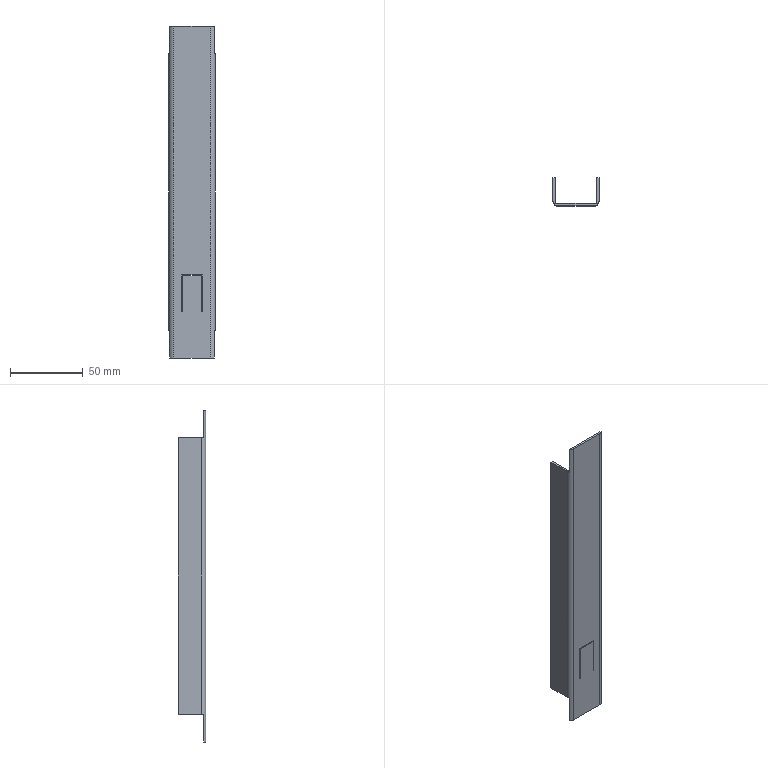Part | SolidWorks | features ICE 2, Extrusion 1 | 1 solid | 26 faces | box 31.75 x 19.05 x 228.6 mm | volume 20094 mm3 | plane 22 | cylinder 4 | commonest cylinder face diameters 3.2 x2 6.4 x2
STEP:
#1=CARTESIAN_POINT('',(31.261,1.5,228.6));
#2=VERTEX_POINT('',#1);
#3=CARTESIAN_POINT('',(0.4889,1.5,228.6));
#4=VERTEX_POINT('',#3);
#5=CARTESIAN_POINT('',(3.1,1.5,228.6));
#6=DIRECTION('',(-1.,0.,0.));
#7=VECTOR('',#6,1000.);
#8=LINE('',#5,#7);
#9=EDGE_CURVE('',#2,#4,#8,.T.);
#10=ORIENTED_EDGE('',*,*,#9,.F.);
#11=CARTESIAN_POINT('',(31.261,1.5,209.55));
#12=VERTEX_POINT('',#11);
#13=CARTESIAN_POINT('',(31.261,1.5,228.6));
#14=DIRECTION('',(0.,0.,-1.));
#15=VECTOR('',#14,1000.);
#16=LINE('',#13,#15);
#17=EDGE_CURVE('',#2,#12,#16,.T.);
#18=ORIENTED_EDGE('',*,*,#17,.T.);
#19=CARTESIAN_POINT('',(28.65,1.5,209.55));
#20=VERTEX_POINT('',#19);
#21=CARTESIAN_POINT('',(31.75,1.5,209.55));
#22=DIRECTION('',(-1.,0.,0.));
#23=VECTOR('',#22,1000.);
#24=LINE('',#21,#23);
#25=EDGE_CURVE('',#12,#20,#24,.T.);
#26=ORIENTED_EDGE('',*,*,#25,.T.);
#27=CARTESIAN_POINT('',(28.65,1.5,19.05));
#28=VERTEX_POINT('',#27);
#29=CARTESIAN_POINT('',(28.65,1.5,228.6));
#30=DIRECTION('',(0.,0.,-1.));
#31=VECTOR('',#30,1000.);
#32=LINE('',#29,#31);
#33=EDGE_CURVE('',#20,#28,#32,.T.);
#34=ORIENTED_EDGE('',*,*,#33,.T.);
#35=CARTESIAN_POINT('',(31.261,1.5,19.05));
#36=VERTEX_POINT('',#35);
#37=CARTESIAN_POINT('',(31.75,1.5,19.05));
#38=DIRECTION('',(-1.,0.,0.));
#39=VECTOR('',#38,1000.);
#40=LINE('',#37,#39);
#41=EDGE_CURVE('',#36,#28,#40,.T.);
#42=ORIENTED_EDGE('',*,*,#41,.F.);
#43=CARTESIAN_POINT('',(31.261,1.5,0.));
#44=VERTEX_POINT('',#43);
#45=CARTESIAN_POINT('',(31.261,1.5,228.6));
#46=DIRECTION('',(0.,0.,-1.));
#47=VECTOR('',#46,1000.);
#48=LINE('',#45,#47);
#49=EDGE_CURVE('',#36,#44,#48,.T.);
#50=ORIENTED_EDGE('',*,*,#49,.T.);
#51=CARTESIAN_POINT('',(0.4889,1.5,0.));
#52=VERTEX_POINT('',#51);
#53=CARTESIAN_POINT('',(3.1,1.5,0.));
#54=DIRECTION('',(-1.,0.,0.));
#55=VECTOR('',#54,1000.);
#56=LINE('',#53,#55);
#57=EDGE_CURVE('',#44,#52,#56,.T.);
#58=ORIENTED_EDGE('',*,*,#57,.T.);
#59=CARTESIAN_POINT('',(0.4889,1.5,19.05));
#60=VERTEX_POINT('',#59);
#61=CARTESIAN_POINT('',(0.4889,1.5,228.6));
#62=DIRECTION('',(0.,0.,1.));
#63=VECTOR('',#62,1000.);
#64=LINE('',#61,#63);
#65=EDGE_CURVE('',#52,#60,#64,.T.);
#66=ORIENTED_EDGE('',*,*,#65,.T.);
#67=CARTESIAN_POINT('',(3.1,1.5,19.05));
#68=VERTEX_POINT('',#67);
#69=CARTESIAN_POINT('',(31.75,1.5,19.05));
#70=DIRECTION('',(-1.,0.,0.));
#71=VECTOR('',#70,1000.);
#72=LINE('',#69,#71);
#73=EDGE_CURVE('',#68,#60,#72,.T.);
#74=ORIENTED_EDGE('',*,*,#73,.F.);
#75=CARTESIAN_POINT('',(3.1,1.5,209.55));
#76=VERTEX_POINT('',#75);
#77=CARTESIAN_POINT('',(3.1,1.5,228.6));
#78=DIRECTION('',(0.,0.,-1.));
#79=VECTOR('',#78,1000.);
#80=LINE('',#77,#79);
#81=EDGE_CURVE('',#76,#68,#80,.T.);
#82=ORIENTED_EDGE('',*,*,#81,.F.);
#83=CARTESIAN_POINT('',(0.4889,1.5,209.55));
#84=VERTEX_POINT('',#83);
#85=CARTESIAN_POINT('',(31.75,1.5,209.55));
#86=DIRECTION('',(-1.,0.,0.));
#87=VECTOR('',#86,1000.);
#88=LINE('',#85,#87);
#89=EDGE_CURVE('',#76,#84,#88,.T.);
#90=ORIENTED_EDGE('',*,*,#89,.T.);
#91=CARTESIAN_POINT('',(0.4889,1.5,228.6));
#92=DIRECTION('',(0.,0.,1.));
#93=VECTOR('',#92,1000.);
#94=LINE('',#91,#93);
#95=EDGE_CURVE('',#84,#4,#94,.T.);
#96=ORIENTED_EDGE('',*,*,#95,.T.);
#97=EDGE_LOOP('',(#10,#18,#26,#34,#42,#50,#58,#66,#74,#82,#90,#96));
#98=FACE_OUTER_BOUND('',#97,.T.);
#99=CARTESIAN_POINT('',(9.428,1.5,31.75));
#100=VERTEX_POINT('',#99);
#101=CARTESIAN_POINT('',(8.928,1.5,31.75));
#102=VERTEX_POINT('',#101);
#103=CARTESIAN_POINT('',(3.1,1.5,31.75));
#104=DIRECTION('',(-1.,0.,0.));
#105=VECTOR('',#104,1000.);
#106=LINE('',#103,#105);
#107=EDGE_CURVE('',#100,#102,#106,.T.);
#108=ORIENTED_EDGE('',*,*,#107,.F.);
#109=CARTESIAN_POINT('',(9.428,1.5,56.65));
#110=VERTEX_POINT('',#109);
#111=CARTESIAN_POINT('',(9.428,1.5,228.6));
#112=DIRECTION('',(0.,0.,-1.));
#113=VECTOR('',#112,1000.);
#114=LINE('',#111,#113);
#115=EDGE_CURVE('',#110,#100,#114,.T.);
#116=ORIENTED_EDGE('',*,*,#115,.F.);
#117=CARTESIAN_POINT('',(22.322,1.5,56.65));
#118=VERTEX_POINT('',#117);
#119=CARTESIAN_POINT('',(3.1,1.5,56.65));
#120=DIRECTION('',(-1.,0.,0.));
#121=VECTOR('',#120,1000.);
#122=LINE('',#119,#121);
#123=EDGE_CURVE('',#118,#110,#122,.T.);
#124=ORIENTED_EDGE('',*,*,#123,.F.);
#125=CARTESIAN_POINT('',(22.322,1.5,31.75));
#126=VERTEX_POINT('',#125);
#127=CARTESIAN_POINT('',(22.322,1.5,228.6));
#128=DIRECTION('',(0.,0.,1.));
#129=VECTOR('',#128,1000.);
#130=LINE('',#127,#129);
#131=EDGE_CURVE('',#126,#118,#130,.T.);
#132=ORIENTED_EDGE('',*,*,#131,.F.);
#133=CARTESIAN_POINT('',(22.822,1.5,31.75));
#134=VERTEX_POINT('',#133);
#135=CARTESIAN_POINT('',(3.1,1.5,31.75));
#136=DIRECTION('',(-1.,0.,0.));
#137=VECTOR('',#136,1000.);
#138=LINE('',#135,#137);
#139=EDGE_CURVE('',#134,#126,#138,.T.);
#140=ORIENTED_EDGE('',*,*,#139,.F.);
#141=CARTESIAN_POINT('',(22.822,1.5,57.15));
#142=VERTEX_POINT('',#141);
#143=CARTESIAN_POINT('',(22.822,1.5,228.6));
#144=DIRECTION('',(0.,0.,-1.));
#145=VECTOR('',#144,1000.);
#146=LINE('',#143,#145);
#147=EDGE_CURVE('',#142,#134,#146,.T.);
#148=ORIENTED_EDGE('',*,*,#147,.F.);
#149=CARTESIAN_POINT('',(8.928,1.5,57.15));
#150=VERTEX_POINT('',#149);
#151=CARTESIAN_POINT('',(3.1,1.5,57.15));
#152=DIRECTION('',(1.,0.,0.));
#153=VECTOR('',#152,1000.);
#154=LINE('',#151,#153);
#155=EDGE_CURVE('',#150,#142,#154,.T.);
#156=ORIENTED_EDGE('',*,*,#155,.F.);
#157=CARTESIAN_POINT('',(8.928,1.5,228.6));
#158=DIRECTION('',(0.,0.,1.));
#159=VECTOR('',#158,1000.);
#160=LINE('',#157,#159);
#161=EDGE_CURVE('',#102,#150,#160,.T.);
#162=ORIENTED_EDGE('',*,*,#161,.F.);
#163=EDGE_LOOP('',(#108,#116,#124,#132,#140,#148,#156,#162));
#164=FACE_BOUND('',#163,.T.);
#165=CARTESIAN_POINT('',(3.1,1.5,228.6));
#166=DIRECTION('',(0.,-1.,0.));
#167=DIRECTION('',(0.,0.,-1.));
#168=AXIS2_PLACEMENT_3D('',#165,#166,#167);
#169=PLANE('',#168);
#170=ADVANCED_FACE('',(#98,#164),#169,.F.);
#171=CARTESIAN_POINT('',(3.2,0.,0.));
#172=VERTEX_POINT('',#171);
#173=CARTESIAN_POINT('',(28.55,0.,0.));
#174=VERTEX_POINT('',#173);
#175=CARTESIAN_POINT('',(3.2,0.,0.));
#176=DIRECTION('',(1.,0.,0.));
#177=VECTOR('',#176,1000.);
#178=LINE('',#175,#177);
#179=EDGE_CURVE('',#172,#174,#178,.T.);
#180=ORIENTED_EDGE('',*,*,#179,.T.);
#181=CARTESIAN_POINT('',(28.55,0.,228.6));
#182=VERTEX_POINT('',#181);
#183=CARTESIAN_POINT('',(28.55,0.,228.6));
#184=DIRECTION('',(0.,0.,-1.));
#185=VECTOR('',#184,1000.);
#186=LINE('',#183,#185);
#187=EDGE_CURVE('',#182,#174,#186,.T.);
#188=ORIENTED_EDGE('',*,*,#187,.F.);
#189=CARTESIAN_POINT('',(3.2,0.,228.6));
#190=VERTEX_POINT('',#189);
#191=CARTESIAN_POINT('',(3.2,0.,228.6));
#192=DIRECTION('',(1.,0.,0.));
#193=VECTOR('',#192,1000.);
#194=LINE('',#191,#193);
#195=EDGE_CURVE('',#190,#182,#194,.T.);
#196=ORIENTED_EDGE('',*,*,#195,.F.);
#197=CARTESIAN_POINT('',(3.2,0.,228.6));
#198=DIRECTION('',(0.,0.,-1.));
#199=VECTOR('',#198,1000.);
#200=LINE('',#197,#199);
#201=EDGE_CURVE('',#190,#172,#200,.T.);
#202=ORIENTED_EDGE('',*,*,#201,.T.);
#203=EDGE_LOOP('',(#180,#188,#196,#202));
#204=FACE_OUTER_BOUND('',#203,.T.);
#205=CARTESIAN_POINT('',(9.428,0.,31.75));
#206=VERTEX_POINT('',#205);
#207=CARTESIAN_POINT('',(8.928,0.,31.75));
#208=VERTEX_POINT('',#207);
#209=CARTESIAN_POINT('',(9.428,0.,31.75));
#210=DIRECTION('',(-1.,0.,0.));
#211=VECTOR('',#210,1000.);
#212=LINE('',#209,#211);
#213=EDGE_CURVE('',#206,#208,#212,.T.);
#214=ORIENTED_EDGE('',*,*,#213,.T.);
#215=CARTESIAN_POINT('',(8.928,0.,57.15));
#216=VERTEX_POINT('',#215);
#217=CARTESIAN_POINT('',(8.928,0.,31.75));
#218=DIRECTION('',(0.,0.,1.));
#219=VECTOR('',#218,1000.);
#220=LINE('',#217,#219);
#221=EDGE_CURVE('',#208,#216,#220,.T.);
#222=ORIENTED_EDGE('',*,*,#221,.T.);
#223=CARTESIAN_POINT('',(22.822,0.,57.15));
#224=VERTEX_POINT('',#223);
#225=CARTESIAN_POINT('',(22.822,0.,57.15));
#226=DIRECTION('',(1.,0.,0.));
#227=VECTOR('',#226,1000.);
#228=LINE('',#225,#227);
#229=EDGE_CURVE('',#216,#224,#228,.T.);
#230=ORIENTED_EDGE('',*,*,#229,.T.);
#231=CARTESIAN_POINT('',(22.822,0.,31.75));
#232=VERTEX_POINT('',#231);
#233=CARTESIAN_POINT('',(22.822,0.,31.75));
#234=DIRECTION('',(0.,0.,-1.));
#235=VECTOR('',#234,1000.);
#236=LINE('',#233,#235);
#237=EDGE_CURVE('',#224,#232,#236,.T.);
#238=ORIENTED_EDGE('',*,*,#237,.T.);
#239=CARTESIAN_POINT('',(22.322,0.,31.75));
#240=VERTEX_POINT('',#239);
#241=CARTESIAN_POINT('',(22.822,0.,31.75));
#242=DIRECTION('',(-1.,0.,0.));
#243=VECTOR('',#242,1000.);
#244=LINE('',#241,#243);
#245=EDGE_CURVE('',#232,#240,#244,.T.);
#246=ORIENTED_EDGE('',*,*,#245,.T.);
#247=CARTESIAN_POINT('',(22.322,0.,56.65));
#248=VERTEX_POINT('',#247);
#249=CARTESIAN_POINT('',(22.322,0.,31.75));
#250=DIRECTION('',(0.,0.,1.));
#251=VECTOR('',#250,1000.);
#252=LINE('',#249,#251);
#253=EDGE_CURVE('',#240,#248,#252,.T.);
#254=ORIENTED_EDGE('',*,*,#253,.T.);
#255=CARTESIAN_POINT('',(9.428,0.,56.65));
#256=VERTEX_POINT('',#255);
#257=CARTESIAN_POINT('',(22.322,0.,56.65));
#258=DIRECTION('',(-1.,0.,0.));
#259=VECTOR('',#258,1000.);
#260=LINE('',#257,#259);
#261=EDGE_CURVE('',#248,#256,#260,.T.);
#262=ORIENTED_EDGE('',*,*,#261,.T.);
#263=CARTESIAN_POINT('',(9.428,0.,31.75));
#264=DIRECTION('',(0.,0.,-1.));
#265=VECTOR('',#264,1000.);
#266=LINE('',#263,#265);
#267=EDGE_CURVE('',#256,#206,#266,.T.);
#268=ORIENTED_EDGE('',*,*,#267,.T.);
#269=EDGE_LOOP('',(#214,#222,#230,#238,#246,#254,#262,#268));
#270=FACE_BOUND('',#269,.T.);
#271=CARTESIAN_POINT('',(3.2,0.,228.6));
#272=DIRECTION('',(0.,1.,0.));
#273=DIRECTION('',(0.,0.,1.));
#274=AXIS2_PLACEMENT_3D('',#271,#272,#273);
#275=PLANE('',#274);
#276=ADVANCED_FACE('',(#204,#270),#275,.F.);
#277=CARTESIAN_POINT('',(31.75,19.05,209.55));
#278=VERTEX_POINT('',#277);
#279=CARTESIAN_POINT('',(30.25,19.05,209.55));
#280=VERTEX_POINT('',#279);
#281=CARTESIAN_POINT('',(31.75,19.05,209.55));
#282=DIRECTION('',(-1.,0.,0.));
#283=VECTOR('',#282,1000.);
#284=LINE('',#281,#283);
#285=EDGE_CURVE('',#278,#280,#284,.T.);
#286=ORIENTED_EDGE('',*,*,#285,.F.);
#287=CARTESIAN_POINT('',(31.75,19.05,19.05));
#288=VERTEX_POINT('',#287);
#289=CARTESIAN_POINT('',(31.75,19.05,228.6));
#290=DIRECTION('',(0.,0.,-1.));
#291=VECTOR('',#290,1000.);
#292=LINE('',#289,#291);
#293=EDGE_CURVE('',#278,#288,#292,.T.);
#294=ORIENTED_EDGE('',*,*,#293,.T.);
#295=CARTESIAN_POINT('',(30.25,19.05,19.05));
#296=VERTEX_POINT('',#295);
#297=CARTESIAN_POINT('',(31.75,19.05,19.05));
#298=DIRECTION('',(-1.,0.,0.));
#299=VECTOR('',#298,1000.);
#300=LINE('',#297,#299);
#301=EDGE_CURVE('',#288,#296,#300,.T.);
#302=ORIENTED_EDGE('',*,*,#301,.T.);
#303=CARTESIAN_POINT('',(30.25,19.05,228.6));
#304=DIRECTION('',(0.,0.,-1.));
#305=VECTOR('',#304,1000.);
#306=LINE('',#303,#305);
#307=EDGE_CURVE('',#280,#296,#306,.T.);
#308=ORIENTED_EDGE('',*,*,#307,.F.);
#309=EDGE_LOOP('',(#286,#294,#302,#308));
#310=FACE_OUTER_BOUND('',#309,.T.);
#311=CARTESIAN_POINT('',(31.75,19.05,228.6));
#312=DIRECTION('',(0.,-1.,0.));
#313=DIRECTION('',(0.,0.,-1.));
#314=AXIS2_PLACEMENT_3D('',#311,#312,#313);
#315=PLANE('',#314);
#316=ADVANCED_FACE('',(#310),#315,.F.);
#317=CARTESIAN_POINT('',(30.25,3.1,209.55));
#318=VERTEX_POINT('',#317);
#319=CARTESIAN_POINT('',(30.25,3.1,209.55));
#320=DIRECTION('',(0.,-1.,0.));
#321=VECTOR('',#320,1000.);
#322=LINE('',#319,#321);
#323=EDGE_CURVE('',#280,#318,#322,.T.);
#324=ORIENTED_EDGE('',*,*,#323,.F.);
#325=ORIENTED_EDGE('',*,*,#307,.T.);
#326=CARTESIAN_POINT('',(30.25,3.1,19.05));
#327=VERTEX_POINT('',#326);
#328=CARTESIAN_POINT('',(30.25,3.1,19.05));
#329=DIRECTION('',(0.,1.,0.));
#330=VECTOR('',#329,1000.);
#331=LINE('',#328,#330);
#332=EDGE_CURVE('',#327,#296,#331,.T.);
#333=ORIENTED_EDGE('',*,*,#332,.F.);
#334=CARTESIAN_POINT('',(30.25,3.1,228.6));
#335=DIRECTION('',(0.,0.,-1.));
#336=VECTOR('',#335,1000.);
#337=LINE('',#334,#336);
#338=EDGE_CURVE('',#318,#327,#337,.T.);
#339=ORIENTED_EDGE('',*,*,#338,.F.);
#340=EDGE_LOOP('',(#324,#325,#333,#339));
#341=FACE_OUTER_BOUND('',#340,.T.);
#342=CARTESIAN_POINT('',(30.25,3.1,228.6));
#343=DIRECTION('',(1.,0.,0.));
#344=DIRECTION('',(0.,1.,0.));
#345=AXIS2_PLACEMENT_3D('',#342,#343,#344);
#346=PLANE('',#345);
#347=ADVANCED_FACE('',(#341),#346,.F.);
#348=CARTESIAN_POINT('',(28.65,3.1,209.55));
#349=DIRECTION('',(0.,0.,-1.));
#350=DIRECTION('',(1.,0.,0.));
#351=AXIS2_PLACEMENT_3D('',#348,#349,#350);
#352=CIRCLE('',#351,1.6);
#353=EDGE_CURVE('',#318,#20,#352,.T.);
#354=ORIENTED_EDGE('',*,*,#353,.F.);
#355=ORIENTED_EDGE('',*,*,#338,.T.);
#356=CARTESIAN_POINT('',(28.65,3.1,19.05));
#357=DIRECTION('',(0.,0.,1.));
#358=DIRECTION('',(0.,1.,0.));
#359=AXIS2_PLACEMENT_3D('',#356,#357,#358);
#360=CIRCLE('',#359,1.6);
#361=EDGE_CURVE('',#28,#327,#360,.T.);
#362=ORIENTED_EDGE('',*,*,#361,.F.);
#363=ORIENTED_EDGE('',*,*,#33,.F.);
#364=EDGE_LOOP('',(#354,#355,#362,#363));
#365=FACE_OUTER_BOUND('',#364,.T.);
#366=CARTESIAN_POINT('',(28.65,3.1,228.6));
#367=DIRECTION('',(0.,0.,-1.));
#368=DIRECTION('',(-1.,0.,0.));
#369=AXIS2_PLACEMENT_3D('',#366,#367,#368);
#370=CYLINDRICAL_SURFACE('',#369,1.6);
#371=ADVANCED_FACE('',(#365),#370,.F.);
#372=CARTESIAN_POINT('',(1.5,3.1,209.55));
#373=VERTEX_POINT('',#372);
#374=CARTESIAN_POINT('',(3.1,3.1,209.55));
#375=DIRECTION('',(0.,0.,-1.));
#376=DIRECTION('',(1.,0.,0.));
#377=AXIS2_PLACEMENT_3D('',#374,#375,#376);
#378=CIRCLE('',#377,1.6);
#379=EDGE_CURVE('',#76,#373,#378,.T.);
#380=ORIENTED_EDGE('',*,*,#379,.F.);
#381=ORIENTED_EDGE('',*,*,#81,.T.);
#382=CARTESIAN_POINT('',(1.5,3.1,19.05));
#383=VERTEX_POINT('',#382);
#384=CARTESIAN_POINT('',(3.1,3.1,19.05));
#385=DIRECTION('',(0.,0.,1.));
#386=DIRECTION('',(0.,1.,0.));
#387=AXIS2_PLACEMENT_3D('',#384,#385,#386);
#388=CIRCLE('',#387,1.6);
#389=EDGE_CURVE('',#383,#68,#388,.T.);
#390=ORIENTED_EDGE('',*,*,#389,.F.);
#391=CARTESIAN_POINT('',(1.5,3.1,228.6));
#392=DIRECTION('',(0.,0.,-1.));
#393=VECTOR('',#392,1000.);
#394=LINE('',#391,#393);
#395=EDGE_CURVE('',#373,#383,#394,.T.);
#396=ORIENTED_EDGE('',*,*,#395,.F.);
#397=EDGE_LOOP('',(#380,#381,#390,#396));
#398=FACE_OUTER_BOUND('',#397,.T.);
#399=CARTESIAN_POINT('',(3.1,3.1,228.6));
#400=DIRECTION('',(0.,0.,-1.));
#401=DIRECTION('',(-1.,0.,0.));
#402=AXIS2_PLACEMENT_3D('',#399,#400,#401);
#403=CYLINDRICAL_SURFACE('',#402,1.6);
#404=ADVANCED_FACE('',(#398),#403,.F.);
#405=CARTESIAN_POINT('',(1.5,19.05,209.55));
#406=VERTEX_POINT('',#405);
#407=CARTESIAN_POINT('',(1.5,3.1,209.55));
#408=DIRECTION('',(0.,1.,0.));
#409=VECTOR('',#408,1000.);
#410=LINE('',#407,#409);
#411=EDGE_CURVE('',#373,#406,#410,.T.);
#412=ORIENTED_EDGE('',*,*,#411,.F.);
#413=ORIENTED_EDGE('',*,*,#395,.T.);
#414=CARTESIAN_POINT('',(1.5,19.05,19.05));
#415=VERTEX_POINT('',#414);
#416=CARTESIAN_POINT('',(1.5,3.1,19.05));
#417=DIRECTION('',(0.,-1.,0.));
#418=VECTOR('',#417,1000.);
#419=LINE('',#416,#418);
#420=EDGE_CURVE('',#415,#383,#419,.T.);
#421=ORIENTED_EDGE('',*,*,#420,.F.);
#422=CARTESIAN_POINT('',(1.5,19.05,228.6));
#423=DIRECTION('',(0.,0.,-1.));
#424=VECTOR('',#423,1000.);
#425=LINE('',#422,#424);
#426=EDGE_CURVE('',#406,#415,#425,.T.);
#427=ORIENTED_EDGE('',*,*,#426,.F.);
#428=EDGE_LOOP('',(#412,#413,#421,#427));
#429=FACE_OUTER_BOUND('',#428,.T.);
#430=CARTESIAN_POINT('',(1.5,3.1,228.6));
#431=DIRECTION('',(-1.,0.,0.));
#432=DIRECTION('',(0.,-1.,0.));
#433=AXIS2_PLACEMENT_3D('',#430,#431,#432);
#434=PLANE('',#433);
#435=ADVANCED_FACE('',(#429),#434,.F.);
#436=CARTESIAN_POINT('',(0.,19.05,209.55));
#437=VERTEX_POINT('',#436);
#438=CARTESIAN_POINT('',(31.75,19.05,209.55));
#439=DIRECTION('',(-1.,0.,0.));
#440=VECTOR('',#439,1000.);
#441=LINE('',#438,#440);
#442=EDGE_CURVE('',#406,#437,#441,.T.);
#443=ORIENTED_EDGE('',*,*,#442,.F.);
#444=ORIENTED_EDGE('',*,*,#426,.T.);
#445=CARTESIAN_POINT('',(0.,19.05,19.05));
#446=VERTEX_POINT('',#445);
#447=CARTESIAN_POINT('',(31.75,19.05,19.05));
#448=DIRECTION('',(-1.,0.,0.));
#449=VECTOR('',#448,1000.);
#450=LINE('',#447,#449);
#451=EDGE_CURVE('',#415,#446,#450,.T.);
#452=ORIENTED_EDGE('',*,*,#451,.T.);
#453=CARTESIAN_POINT('',(0.,19.05,228.6));
#454=DIRECTION('',(0.,0.,-1.));
#455=VECTOR('',#454,1000.);
#456=LINE('',#453,#455);
#457=EDGE_CURVE('',#437,#446,#456,.T.);
#458=ORIENTED_EDGE('',*,*,#457,.F.);
#459=EDGE_LOOP('',(#443,#444,#452,#458));
#460=FACE_OUTER_BOUND('',#459,.T.);
#461=CARTESIAN_POINT('',(1.5,19.05,228.6));
#462=DIRECTION('',(0.,-1.,0.));
#463=DIRECTION('',(0.,0.,-1.));
#464=AXIS2_PLACEMENT_3D('',#461,#462,#463);
#465=PLANE('',#464);
#466=ADVANCED_FACE('',(#460),#465,.F.);
#467=CARTESIAN_POINT('',(0.,3.2,209.55));
#468=VERTEX_POINT('',#467);
#469=CARTESIAN_POINT('',(0.,1.5,209.55));
#470=DIRECTION('',(0.,1.,0.));
#471=VECTOR('',#470,1000.);
#472=LINE('',#469,#471);
#473=EDGE_CURVE('',#468,#437,#472,.T.);
#474=ORIENTED_EDGE('',*,*,#473,.T.);
#475=ORIENTED_EDGE('',*,*,#457,.T.);
#476=CARTESIAN_POINT('',(0.,3.2,19.05));
#477=VERTEX_POINT('',#476);
#478=CARTESIAN_POINT('',(0.,1.5,19.05));
#479=DIRECTION('',(0.,-1.,0.));
#480=VECTOR('',#479,1000.);
#481=LINE('',#478,#480);
#482=EDGE_CURVE('',#446,#477,#481,.T.);
#483=ORIENTED_EDGE('',*,*,#482,.T.);
#484=CARTESIAN_POINT('',(0.,3.2,228.6));
#485=DIRECTION('',(0.,0.,-1.));
#486=VECTOR('',#485,1000.);
#487=LINE('',#484,#486);
#488=EDGE_CURVE('',#468,#477,#487,.T.);
#489=ORIENTED_EDGE('',*,*,#488,.F.);
#490=EDGE_LOOP('',(#474,#475,#483,#489));
#491=FACE_OUTER_BOUND('',#490,.T.);
#492=CARTESIAN_POINT('',(0.,3.2,228.6));
#493=DIRECTION('',(1.,0.,0.));
#494=DIRECTION('',(0.,0.,-1.));
#495=AXIS2_PLACEMENT_3D('',#492,#493,#494);
#496=PLANE('',#495);
#497=ADVANCED_FACE('',(#491),#496,.F.);
#498=ORIENTED_EDGE('',*,*,#95,.F.);
#499=CARTESIAN_POINT('',(3.2,3.2,209.55));
#500=DIRECTION('',(0.,0.,1.));
#501=DIRECTION('',(1.,0.,0.));
#502=AXIS2_PLACEMENT_3D('',#499,#500,#501);
#503=CIRCLE('',#502,3.2);
#504=EDGE_CURVE('',#468,#84,#503,.T.);
#505=ORIENTED_EDGE('',*,*,#504,.F.);
#506=ORIENTED_EDGE('',*,*,#488,.T.);
#507=CARTESIAN_POINT('',(3.2,3.2,19.05));
#508=DIRECTION('',(0.,0.,-1.));
#509=DIRECTION('',(0.,1.,0.));
#510=AXIS2_PLACEMENT_3D('',#507,#508,#509);
#511=CIRCLE('',#510,3.2);
#512=EDGE_CURVE('',#60,#477,#511,.T.);
#513=ORIENTED_EDGE('',*,*,#512,.F.);
#514=ORIENTED_EDGE('',*,*,#65,.F.);
#515=CARTESIAN_POINT('',(3.2,3.2,0.));
#516=DIRECTION('',(0.,0.,1.));
#517=DIRECTION('',(1.,0.,0.));
#518=AXIS2_PLACEMENT_3D('',#515,#516,#517);
#519=CIRCLE('',#518,3.2);
#520=EDGE_CURVE('',#52,#172,#519,.T.);
#521=ORIENTED_EDGE('',*,*,#520,.T.);
#522=ORIENTED_EDGE('',*,*,#201,.F.);
#523=CARTESIAN_POINT('',(3.2,3.2,228.6));
#524=DIRECTION('',(0.,0.,1.));
#525=DIRECTION('',(1.,0.,0.));
#526=AXIS2_PLACEMENT_3D('',#523,#524,#525);
#527=CIRCLE('',#526,3.2);
#528=EDGE_CURVE('',#4,#190,#527,.T.);
#529=ORIENTED_EDGE('',*,*,#528,.F.);
#530=EDGE_LOOP('',(#498,#505,#506,#513,#514,#521,#522,#529));
#531=FACE_OUTER_BOUND('',#530,.T.);
#532=CARTESIAN_POINT('',(3.2,3.2,228.6));
#533=DIRECTION('',(0.,0.,-1.));
#534=DIRECTION('',(-1.,0.,0.));
#535=AXIS2_PLACEMENT_3D('',#532,#533,#534);
#536=CYLINDRICAL_SURFACE('',#535,3.2);
#537=ADVANCED_FACE('',(#531),#536,.T.);
#538=ORIENTED_EDGE('',*,*,#17,.F.);
#539=CARTESIAN_POINT('',(28.55,3.2,228.6));
#540=DIRECTION('',(0.,0.,1.));
#541=DIRECTION('',(-1.,0.,0.));
#542=AXIS2_PLACEMENT_3D('',#539,#540,#541);
#543=CIRCLE('',#542,3.2);
#544=EDGE_CURVE('',#182,#2,#543,.T.);
#545=ORIENTED_EDGE('',*,*,#544,.F.);
#546=ORIENTED_EDGE('',*,*,#187,.T.);
#547=CARTESIAN_POINT('',(28.55,3.2,0.));
#548=DIRECTION('',(0.,0.,1.));
#549=DIRECTION('',(-1.,0.,0.));
#550=AXIS2_PLACEMENT_3D('',#547,#548,#549);
#551=CIRCLE('',#550,3.2);
#552=EDGE_CURVE('',#174,#44,#551,.T.);
#553=ORIENTED_EDGE('',*,*,#552,.T.);
#554=ORIENTED_EDGE('',*,*,#49,.F.);
#555=CARTESIAN_POINT('',(31.75,3.2,19.05));
#556=VERTEX_POINT('',#555);
#557=CARTESIAN_POINT('',(28.55,3.2,19.05));
#558=DIRECTION('',(0.,0.,-1.));
#559=DIRECTION('',(0.,1.,0.));
#560=AXIS2_PLACEMENT_3D('',#557,#558,#559);
#561=CIRCLE('',#560,3.2);
#562=EDGE_CURVE('',#556,#36,#561,.T.);
#563=ORIENTED_EDGE('',*,*,#562,.F.);
#564=CARTESIAN_POINT('',(31.75,3.2,209.55));
#565=VERTEX_POINT('',#564);
#566=CARTESIAN_POINT('',(31.75,3.2,228.6));
#567=DIRECTION('',(0.,0.,-1.));
#568=VECTOR('',#567,1000.);
#569=LINE('',#566,#568);
#570=EDGE_CURVE('',#565,#556,#569,.T.);
#571=ORIENTED_EDGE('',*,*,#570,.F.);
#572=CARTESIAN_POINT('',(28.55,3.2,209.55));
#573=DIRECTION('',(0.,0.,1.));
#574=DIRECTION('',(1.,0.,0.));
#575=AXIS2_PLACEMENT_3D('',#572,#573,#574);
#576=CIRCLE('',#575,3.2);
#577=EDGE_CURVE('',#12,#565,#576,.T.);
#578=ORIENTED_EDGE('',*,*,#577,.F.);
#579=EDGE_LOOP('',(#538,#545,#546,#553,#554,#563,#571,#578));
#580=FACE_OUTER_BOUND('',#579,.T.);
#581=CARTESIAN_POINT('',(28.55,3.2,228.6));
#582=DIRECTION('',(0.,0.,-1.));
#583=DIRECTION('',(-1.,0.,0.));
#584=AXIS2_PLACEMENT_3D('',#581,#582,#583);
#585=CYLINDRICAL_SURFACE('',#584,3.2);
#586=ADVANCED_FACE('',(#580),#585,.T.);
#587=CARTESIAN_POINT('',(31.75,1.5,209.55));
#588=DIRECTION('',(0.,1.,0.));
#589=VECTOR('',#588,1000.);
#590=LINE('',#587,#589);
#591=EDGE_CURVE('',#565,#278,#590,.T.);
#592=ORIENTED_EDGE('',*,*,#591,.F.);
#593=ORIENTED_EDGE('',*,*,#570,.T.);
#594=CARTESIAN_POINT('',(31.75,1.5,19.05));
#595=DIRECTION('',(0.,-1.,0.));
#596=VECTOR('',#595,1000.);
#597=LINE('',#594,#596);
#598=EDGE_CURVE('',#288,#556,#597,.T.);
#599=ORIENTED_EDGE('',*,*,#598,.F.);
#600=ORIENTED_EDGE('',*,*,#293,.F.);
#601=EDGE_LOOP('',(#592,#593,#599,#600));
#602=FACE_OUTER_BOUND('',#601,.T.);
#603=CARTESIAN_POINT('',(31.75,3.2,228.6));
#604=DIRECTION('',(-1.,0.,0.));
#605=DIRECTION('',(0.,0.,1.));
#606=AXIS2_PLACEMENT_3D('',#603,#604,#605);
#607=PLANE('',#606);
#608=ADVANCED_FACE('',(#602),#607,.F.);
#609=ORIENTED_EDGE('',*,*,#544,.T.);
#610=ORIENTED_EDGE('',*,*,#9,.T.);
#611=ORIENTED_EDGE('',*,*,#528,.T.);
#612=ORIENTED_EDGE('',*,*,#195,.T.);
#613=EDGE_LOOP('',(#609,#610,#611,#612));
#614=FACE_OUTER_BOUND('',#613,.T.);
#615=CARTESIAN_POINT('',(28.65,3.1,228.6));
#616=DIRECTION('',(0.,0.,1.));
#617=DIRECTION('',(1.,0.,0.));
#618=AXIS2_PLACEMENT_3D('',#615,#616,#617);
#619=PLANE('',#618);
#620=ADVANCED_FACE('',(#614),#619,.T.);
#621=ORIENTED_EDGE('',*,*,#57,.F.);
#622=ORIENTED_EDGE('',*,*,#552,.F.);
#623=ORIENTED_EDGE('',*,*,#179,.F.);
#624=ORIENTED_EDGE('',*,*,#520,.F.);
#625=EDGE_LOOP('',(#621,#622,#623,#624));
#626=FACE_OUTER_BOUND('',#625,.T.);
#627=CARTESIAN_POINT('',(28.65,3.1,0.));
#628=DIRECTION('',(0.,0.,1.));
#629=DIRECTION('',(1.,0.,0.));
#630=AXIS2_PLACEMENT_3D('',#627,#628,#629);
#631=PLANE('',#630);
#632=ADVANCED_FACE('',(#626),#631,.F.);
#633=ORIENTED_EDGE('',*,*,#389,.T.);
#634=ORIENTED_EDGE('',*,*,#73,.T.);
#635=ORIENTED_EDGE('',*,*,#512,.T.);
#636=ORIENTED_EDGE('',*,*,#482,.F.);
#637=ORIENTED_EDGE('',*,*,#451,.F.);
#638=ORIENTED_EDGE('',*,*,#420,.T.);
#639=EDGE_LOOP('',(#633,#634,#635,#636,#637,#638));
#640=FACE_OUTER_BOUND('',#639,.T.);
#641=CARTESIAN_POINT('',(31.75,1.5,19.05));
#642=DIRECTION('',(0.,0.,-1.));
#643=DIRECTION('',(0.,1.,0.));
#644=AXIS2_PLACEMENT_3D('',#641,#642,#643);
#645=PLANE('',#644);
#646=ADVANCED_FACE('',(#640),#645,.T.);
#647=ORIENTED_EDGE('',*,*,#332,.T.);
#648=ORIENTED_EDGE('',*,*,#301,.F.);
#649=ORIENTED_EDGE('',*,*,#598,.T.);
#650=ORIENTED_EDGE('',*,*,#562,.T.);
#651=ORIENTED_EDGE('',*,*,#41,.T.);
#652=ORIENTED_EDGE('',*,*,#361,.T.);
#653=EDGE_LOOP('',(#647,#648,#649,#650,#651,#652));
#654=FACE_OUTER_BOUND('',#653,.T.);
#655=CARTESIAN_POINT('',(31.75,1.5,19.05));
#656=DIRECTION('',(0.,0.,-1.));
#657=DIRECTION('',(0.,1.,0.));
#658=AXIS2_PLACEMENT_3D('',#655,#656,#657);
#659=PLANE('',#658);
#660=ADVANCED_FACE('',(#654),#659,.T.);
#661=ORIENTED_EDGE('',*,*,#379,.T.);
#662=ORIENTED_EDGE('',*,*,#411,.T.);
#663=ORIENTED_EDGE('',*,*,#442,.T.);
#664=ORIENTED_EDGE('',*,*,#473,.F.);
#665=ORIENTED_EDGE('',*,*,#504,.T.);
#666=ORIENTED_EDGE('',*,*,#89,.F.);
#667=EDGE_LOOP('',(#661,#662,#663,#664,#665,#666));
#668=FACE_OUTER_BOUND('',#667,.T.);
#669=CARTESIAN_POINT('',(31.75,1.5,209.55));
#670=DIRECTION('',(0.,0.,1.));
#671=DIRECTION('',(1.,0.,0.));
#672=AXIS2_PLACEMENT_3D('',#669,#670,#671);
#673=PLANE('',#672);
#674=ADVANCED_FACE('',(#668),#673,.T.);
#675=ORIENTED_EDGE('',*,*,#323,.T.);
#676=ORIENTED_EDGE('',*,*,#353,.T.);
#677=ORIENTED_EDGE('',*,*,#25,.F.);
#678=ORIENTED_EDGE('',*,*,#577,.T.);
#679=ORIENTED_EDGE('',*,*,#591,.T.);
#680=ORIENTED_EDGE('',*,*,#285,.T.);
#681=EDGE_LOOP('',(#675,#676,#677,#678,#679,#680));
#682=FACE_OUTER_BOUND('',#681,.T.);
#683=CARTESIAN_POINT('',(31.75,1.5,209.55));
#684=DIRECTION('',(0.,0.,1.));
#685=DIRECTION('',(1.,0.,0.));
#686=AXIS2_PLACEMENT_3D('',#683,#684,#685);
#687=PLANE('',#686);
#688=ADVANCED_FACE('',(#682),#687,.T.);
#689=ORIENTED_EDGE('',*,*,#107,.T.);
#690=CARTESIAN_POINT('',(8.928,19.05,31.75));
#691=DIRECTION('',(0.,-1.,0.));
#692=VECTOR('',#691,1000.);
#693=LINE('',#690,#692);
#694=EDGE_CURVE('',#102,#208,#693,.T.);
#695=ORIENTED_EDGE('',*,*,#694,.T.);
#696=ORIENTED_EDGE('',*,*,#213,.F.);
#697=CARTESIAN_POINT('',(9.428,19.05,31.75));
#698=DIRECTION('',(0.,-1.,0.));
#699=VECTOR('',#698,1000.);
#700=LINE('',#697,#699);
#701=EDGE_CURVE('',#100,#206,#700,.T.);
#702=ORIENTED_EDGE('',*,*,#701,.F.);
#703=EDGE_LOOP('',(#689,#695,#696,#702));
#704=FACE_OUTER_BOUND('',#703,.T.);
#705=CARTESIAN_POINT('',(9.428,19.05,31.75));
#706=DIRECTION('',(0.,0.,1.));
#707=DIRECTION('',(1.,0.,0.));
#708=AXIS2_PLACEMENT_3D('',#705,#706,#707);
#709=PLANE('',#708);
#710=ADVANCED_FACE('',(#704),#709,.T.);
#711=ORIENTED_EDGE('',*,*,#161,.T.);
#712=CARTESIAN_POINT('',(8.928,19.05,57.15));
#713=DIRECTION('',(0.,-1.,0.));
#714=VECTOR('',#713,1000.);
#715=LINE('',#712,#714);
#716=EDGE_CURVE('',#150,#216,#715,.T.);
#717=ORIENTED_EDGE('',*,*,#716,.T.);
#718=ORIENTED_EDGE('',*,*,#221,.F.);
#719=ORIENTED_EDGE('',*,*,#694,.F.);
#720=EDGE_LOOP('',(#711,#717,#718,#719));
#721=FACE_OUTER_BOUND('',#720,.T.);
#722=CARTESIAN_POINT('',(8.928,19.05,31.75));
#723=DIRECTION('',(1.,0.,0.));
#724=DIRECTION('',(0.,0.,-1.));
#725=AXIS2_PLACEMENT_3D('',#722,#723,#724);
#726=PLANE('',#725);
#727=ADVANCED_FACE('',(#721),#726,.T.);
#728=ORIENTED_EDGE('',*,*,#155,.T.);
#729=CARTESIAN_POINT('',(22.822,19.05,57.15));
#730=DIRECTION('',(0.,-1.,0.));
#731=VECTOR('',#730,1000.);
#732=LINE('',#729,#731);
#733=EDGE_CURVE('',#142,#224,#732,.T.);
#734=ORIENTED_EDGE('',*,*,#733,.T.);
#735=ORIENTED_EDGE('',*,*,#229,.F.);
#736=ORIENTED_EDGE('',*,*,#716,.F.);
#737=EDGE_LOOP('',(#728,#734,#735,#736));
#738=FACE_OUTER_BOUND('',#737,.T.);
#739=CARTESIAN_POINT('',(22.822,19.05,57.15));
#740=DIRECTION('',(0.,0.,-1.));
#741=DIRECTION('',(-1.,0.,0.));
#742=AXIS2_PLACEMENT_3D('',#739,#740,#741);
#743=PLANE('',#742);
#744=ADVANCED_FACE('',(#738),#743,.T.);
#745=ORIENTED_EDGE('',*,*,#147,.T.);
#746=CARTESIAN_POINT('',(22.822,19.05,31.75));
#747=DIRECTION('',(0.,-1.,0.));
#748=VECTOR('',#747,1000.);
#749=LINE('',#746,#748);
#750=EDGE_CURVE('',#134,#232,#749,.T.);
#751=ORIENTED_EDGE('',*,*,#750,.T.);
#752=ORIENTED_EDGE('',*,*,#237,.F.);
#753=ORIENTED_EDGE('',*,*,#733,.F.);
#754=EDGE_LOOP('',(#745,#751,#752,#753));
#755=FACE_OUTER_BOUND('',#754,.T.);
#756=CARTESIAN_POINT('',(22.822,19.05,31.75));
#757=DIRECTION('',(-1.,0.,0.));
#758=DIRECTION('',(0.,0.,1.));
#759=AXIS2_PLACEMENT_3D('',#756,#757,#758);
#760=PLANE('',#759);
#761=ADVANCED_FACE('',(#755),#760,.T.);
#762=ORIENTED_EDGE('',*,*,#139,.T.);
#763=CARTESIAN_POINT('',(22.322,19.05,31.75));
#764=DIRECTION('',(0.,-1.,0.));
#765=VECTOR('',#764,1000.);
#766=LINE('',#763,#765);
#767=EDGE_CURVE('',#126,#240,#766,.T.);
#768=ORIENTED_EDGE('',*,*,#767,.T.);
#769=ORIENTED_EDGE('',*,*,#245,.F.);
#770=ORIENTED_EDGE('',*,*,#750,.F.);
#771=EDGE_LOOP('',(#762,#768,#769,#770));
#772=FACE_OUTER_BOUND('',#771,.T.);
#773=CARTESIAN_POINT('',(22.822,19.05,31.75));
#774=DIRECTION('',(0.,0.,1.));
#775=DIRECTION('',(1.,0.,0.));
#776=AXIS2_PLACEMENT_3D('',#773,#774,#775);
#777=PLANE('',#776);
#778=ADVANCED_FACE('',(#772),#777,.T.);
#779=ORIENTED_EDGE('',*,*,#131,.T.);
#780=CARTESIAN_POINT('',(22.322,19.05,56.65));
#781=DIRECTION('',(0.,-1.,0.));
#782=VECTOR('',#781,1000.);
#783=LINE('',#780,#782);
#784=EDGE_CURVE('',#118,#248,#783,.T.);
#785=ORIENTED_EDGE('',*,*,#784,.T.);
#786=ORIENTED_EDGE('',*,*,#253,.F.);
#787=ORIENTED_EDGE('',*,*,#767,.F.);
#788=EDGE_LOOP('',(#779,#785,#786,#787));
#789=FACE_OUTER_BOUND('',#788,.T.);
#790=CARTESIAN_POINT('',(22.322,19.05,31.75));
#791=DIRECTION('',(1.,0.,0.));
#792=DIRECTION('',(0.,0.,-1.));
#793=AXIS2_PLACEMENT_3D('',#790,#791,#792);
#794=PLANE('',#793);
#795=ADVANCED_FACE('',(#789),#794,.T.);
#796=ORIENTED_EDGE('',*,*,#123,.T.);
#797=CARTESIAN_POINT('',(9.428,19.05,56.65));
#798=DIRECTION('',(0.,-1.,0.));
#799=VECTOR('',#798,1000.);
#800=LINE('',#797,#799);
#801=EDGE_CURVE('',#110,#256,#800,.T.);
#802=ORIENTED_EDGE('',*,*,#801,.T.);
#803=ORIENTED_EDGE('',*,*,#261,.F.);
#804=ORIENTED_EDGE('',*,*,#784,.F.);
#805=EDGE_LOOP('',(#796,#802,#803,#804));
#806=FACE_OUTER_BOUND('',#805,.T.);
#807=CARTESIAN_POINT('',(22.322,19.05,56.65));
#808=DIRECTION('',(0.,0.,1.));
#809=DIRECTION('',(1.,0.,0.));
#810=AXIS2_PLACEMENT_3D('',#807,#808,#809);
#811=PLANE('',#810);
#812=ADVANCED_FACE('',(#806),#811,.T.);
#813=ORIENTED_EDGE('',*,*,#115,.T.);
#814=ORIENTED_EDGE('',*,*,#701,.T.);
#815=ORIENTED_EDGE('',*,*,#267,.F.);
#816=ORIENTED_EDGE('',*,*,#801,.F.);
#817=EDGE_LOOP('',(#813,#814,#815,#816));
#818=FACE_OUTER_BOUND('',#817,.T.);
#819=CARTESIAN_POINT('',(9.428,19.05,31.75));
#820=DIRECTION('',(-1.,0.,0.));
#821=DIRECTION('',(0.,0.,1.));
#822=AXIS2_PLACEMENT_3D('',#819,#820,#821);
#823=PLANE('',#822);
#824=ADVANCED_FACE('',(#818),#823,.T.);
#825=CLOSED_SHELL('',(#170,#276,#316,#347,#371,#404,#435,#466,#497,#537,#586,#608,#620,#632,#646,#660,#674,#688,#710,#727,#744,#761,#778,#795,#812,#824));
#826=MANIFOLD_SOLID_BREP('',#825);
#827=CARTESIAN_POINT('',(0.,0.,0.));
#828=DIRECTION('',(0.,0.,1.));
#829=DIRECTION('',(1.,0.,0.));
#830=AXIS2_PLACEMENT_3D('',#827,#828,#829);
#831=(LENGTH_UNIT()NAMED_UNIT(*)SI_UNIT(.MILLI.,.METRE.));
#832=UNCERTAINTY_MEASURE_WITH_UNIT(LENGTH_MEASURE(0.00001),#831,'','');
#833=(NAMED_UNIT(*)PLANE_ANGLE_UNIT()SI_UNIT($,.RADIAN.));
#834=(NAMED_UNIT(*)SI_UNIT($,.STERADIAN.)SOLID_ANGLE_UNIT());
#835=(GEOMETRIC_REPRESENTATION_CONTEXT(3)GLOBAL_UNCERTAINTY_ASSIGNED_CONTEXT((#832))GLOBAL_UNIT_ASSIGNED_CONTEXT((#831,#833,#834))REPRESENTATION_CONTEXT('',''));
#836=ADVANCED_BREP_SHAPE_REPRESENTATION('',(#826,#830),#835);